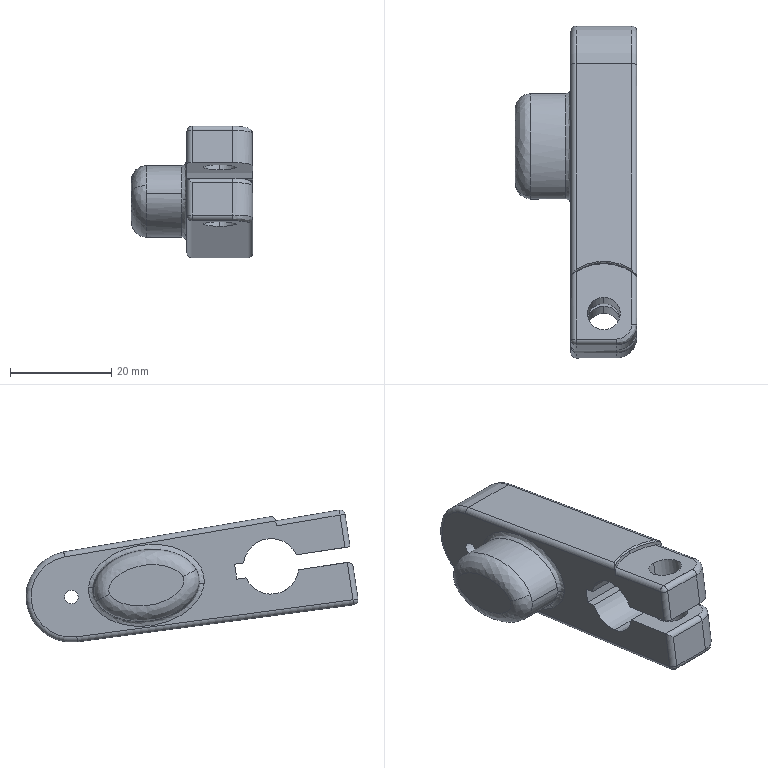Part | SolidWorks | features BaseBody 1 | 1 solid | 62 faces | box 24 x 65.725 x 26.174 mm | volume 14700 mm3 | cylinder 30 | plane 13 | spline 8 | cone 4 | torus 4 | sphere 3 | commonest cylinder face diameters 2 x14 6 x4 6.5 x4 11 x3 8 x2 20 x2